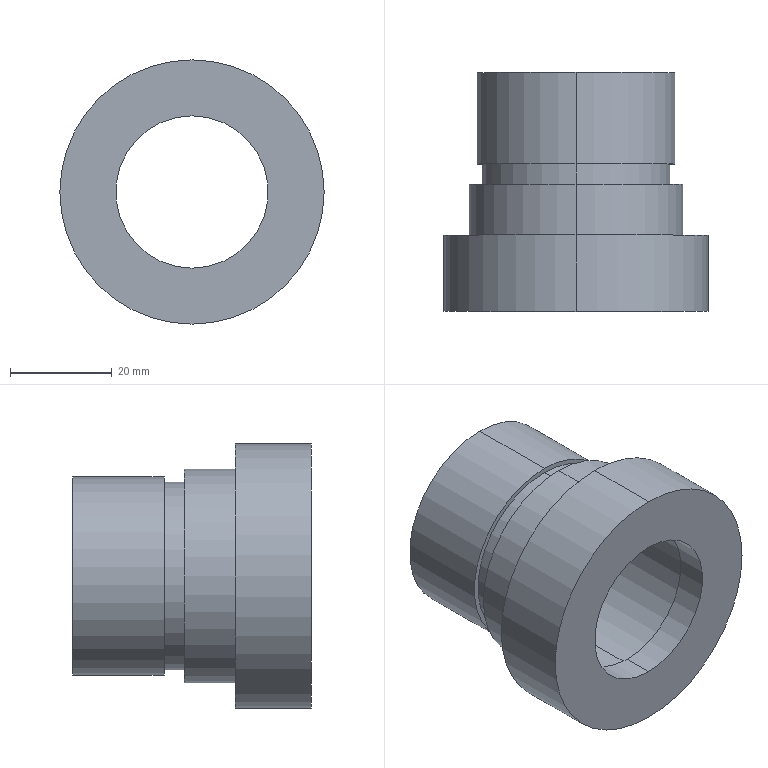Part | SolidWorks | features BaseBody 1 | 1 solid | 24 faces | box 52 x 47 x 52 mm | volume 34093 mm3 | cylinder 16 | plane 8 | commonest cylinder face diameters 32 x4 30 x2 35 x2 37 x2 39 x2 42 x2
STEP:
#1=CARTESIAN_POINT('',(0.,6.,-16.));
#2=VERTEX_POINT('',#1);
#3=CARTESIAN_POINT('',(0.,6.,16.));
#4=VERTEX_POINT('',#3);
#5=CARTESIAN_POINT('',(0.,6.,0.));
#6=DIRECTION('',(0.,1.,0.));
#7=DIRECTION('',(0.,0.,1.));
#8=AXIS2_PLACEMENT_3D('',#5,#6,#7);
#9=CIRCLE('',#8,16.);
#10=EDGE_CURVE('',#2,#4,#9,.T.);
#11=ORIENTED_EDGE('',*,*,#10,.F.);
#12=CARTESIAN_POINT('',(0.,41.,-16.));
#13=VERTEX_POINT('',#12);
#14=CARTESIAN_POINT('',(0.,6.,-16.));
#15=DIRECTION('',(0.,1.,0.));
#16=VECTOR('',#15,1000.);
#17=LINE('',#14,#16);
#18=EDGE_CURVE('',#2,#13,#17,.T.);
#19=ORIENTED_EDGE('',*,*,#18,.T.);
#20=CARTESIAN_POINT('',(0.,41.,16.));
#21=VERTEX_POINT('',#20);
#22=CARTESIAN_POINT('',(0.,41.,0.));
#23=DIRECTION('',(0.,-1.,0.));
#24=DIRECTION('',(0.,0.,1.));
#25=AXIS2_PLACEMENT_3D('',#22,#23,#24);
#26=CIRCLE('',#25,16.);
#27=EDGE_CURVE('',#21,#13,#26,.T.);
#28=ORIENTED_EDGE('',*,*,#27,.F.);
#29=CARTESIAN_POINT('',(0.,6.,16.));
#30=DIRECTION('',(0.,1.,0.));
#31=VECTOR('',#30,1000.);
#32=LINE('',#29,#31);
#33=EDGE_CURVE('',#4,#21,#32,.T.);
#34=ORIENTED_EDGE('',*,*,#33,.F.);
#35=EDGE_LOOP('',(#11,#19,#28,#34));
#36=FACE_OUTER_BOUND('',#35,.T.);
#37=CARTESIAN_POINT('',(0.,6.,0.));
#38=DIRECTION('',(0.,1.,0.));
#39=DIRECTION('',(0.,0.,1.));
#40=AXIS2_PLACEMENT_3D('',#37,#38,#39);
#41=CYLINDRICAL_SURFACE('',#40,16.);
#42=ADVANCED_FACE('',(#36),#41,.F.);
#43=CARTESIAN_POINT('',(0.,6.,15.));
#44=VERTEX_POINT('',#43);
#45=CARTESIAN_POINT('',(0.,6.,-15.));
#46=VERTEX_POINT('',#45);
#47=CARTESIAN_POINT('',(0.,6.,0.));
#48=DIRECTION('',(0.,-1.,0.));
#49=DIRECTION('',(0.,0.,-1.));
#50=AXIS2_PLACEMENT_3D('',#47,#48,#49);
#51=CIRCLE('',#50,15.);
#52=EDGE_CURVE('',#44,#46,#51,.T.);
#53=ORIENTED_EDGE('',*,*,#52,.F.);
#54=CARTESIAN_POINT('',(0.,0.,15.));
#55=VERTEX_POINT('',#54);
#56=CARTESIAN_POINT('',(0.,47.,15.));
#57=DIRECTION('',(0.,-1.,0.));
#58=VECTOR('',#57,1000.);
#59=LINE('',#56,#58);
#60=EDGE_CURVE('',#44,#55,#59,.T.);
#61=ORIENTED_EDGE('',*,*,#60,.T.);
#62=CARTESIAN_POINT('',(0.,0.,-15.));
#63=VERTEX_POINT('',#62);
#64=CARTESIAN_POINT('',(0.,0.,0.));
#65=DIRECTION('',(0.,1.,0.));
#66=DIRECTION('',(0.,0.,-1.));
#67=AXIS2_PLACEMENT_3D('',#64,#65,#66);
#68=CIRCLE('',#67,15.);
#69=EDGE_CURVE('',#63,#55,#68,.T.);
#70=ORIENTED_EDGE('',*,*,#69,.F.);
#71=CARTESIAN_POINT('',(0.,47.,-15.));
#72=DIRECTION('',(0.,-1.,0.));
#73=VECTOR('',#72,1000.);
#74=LINE('',#71,#73);
#75=EDGE_CURVE('',#46,#63,#74,.T.);
#76=ORIENTED_EDGE('',*,*,#75,.F.);
#77=EDGE_LOOP('',(#53,#61,#70,#76));
#78=FACE_OUTER_BOUND('',#77,.T.);
#79=CARTESIAN_POINT('',(0.,47.,0.));
#80=DIRECTION('',(0.,-1.,0.));
#81=DIRECTION('',(0.,0.,-1.));
#82=AXIS2_PLACEMENT_3D('',#79,#80,#81);
#83=CYLINDRICAL_SURFACE('',#82,15.);
#84=ADVANCED_FACE('',(#78),#83,.F.);
#85=CARTESIAN_POINT('',(0.,42.3,17.5));
#86=VERTEX_POINT('',#85);
#87=CARTESIAN_POINT('',(0.,42.3,-17.5));
#88=VERTEX_POINT('',#87);
#89=CARTESIAN_POINT('',(0.,42.3,0.));
#90=DIRECTION('',(0.,-1.,0.));
#91=DIRECTION('',(0.,0.,-1.));
#92=AXIS2_PLACEMENT_3D('',#89,#90,#91);
#93=CIRCLE('',#92,17.5);
#94=EDGE_CURVE('',#86,#88,#93,.T.);
#95=ORIENTED_EDGE('',*,*,#94,.F.);
#96=CARTESIAN_POINT('',(0.,41.,17.5));
#97=VERTEX_POINT('',#96);
#98=CARTESIAN_POINT('',(0.,42.3,17.5));
#99=DIRECTION('',(0.,-1.,0.));
#100=VECTOR('',#99,1000.);
#101=LINE('',#98,#100);
#102=EDGE_CURVE('',#86,#97,#101,.T.);
#103=ORIENTED_EDGE('',*,*,#102,.T.);
#104=CARTESIAN_POINT('',(0.,41.,-17.5));
#105=VERTEX_POINT('',#104);
#106=CARTESIAN_POINT('',(0.,41.,0.));
#107=DIRECTION('',(0.,1.,0.));
#108=DIRECTION('',(0.,0.,-1.));
#109=AXIS2_PLACEMENT_3D('',#106,#107,#108);
#110=CIRCLE('',#109,17.5);
#111=EDGE_CURVE('',#105,#97,#110,.T.);
#112=ORIENTED_EDGE('',*,*,#111,.F.);
#113=CARTESIAN_POINT('',(0.,42.3,-17.5));
#114=DIRECTION('',(0.,-1.,0.));
#115=VECTOR('',#114,1000.);
#116=LINE('',#113,#115);
#117=EDGE_CURVE('',#88,#105,#116,.T.);
#118=ORIENTED_EDGE('',*,*,#117,.F.);
#119=EDGE_LOOP('',(#95,#103,#112,#118));
#120=FACE_OUTER_BOUND('',#119,.T.);
#121=CARTESIAN_POINT('',(0.,42.3,0.));
#122=DIRECTION('',(0.,-1.,0.));
#123=DIRECTION('',(0.,0.,-1.));
#124=AXIS2_PLACEMENT_3D('',#121,#122,#123);
#125=CYLINDRICAL_SURFACE('',#124,17.5);
#126=ADVANCED_FACE('',(#120),#125,.F.);
#127=CARTESIAN_POINT('',(0.,15.,-26.));
#128=VERTEX_POINT('',#127);
#129=CARTESIAN_POINT('',(0.,15.,26.));
#130=VERTEX_POINT('',#129);
#131=CARTESIAN_POINT('',(0.,15.,0.));
#132=DIRECTION('',(0.,-1.,0.));
#133=DIRECTION('',(0.,0.,-1.));
#134=AXIS2_PLACEMENT_3D('',#131,#132,#133);
#135=CIRCLE('',#134,26.);
#136=EDGE_CURVE('',#128,#130,#135,.T.);
#137=ORIENTED_EDGE('',*,*,#136,.T.);
#138=CARTESIAN_POINT('',(0.,0.,26.));
#139=VERTEX_POINT('',#138);
#140=CARTESIAN_POINT('',(0.,47.,26.));
#141=DIRECTION('',(0.,-1.,0.));
#142=VECTOR('',#141,1000.);
#143=LINE('',#140,#142);
#144=EDGE_CURVE('',#130,#139,#143,.T.);
#145=ORIENTED_EDGE('',*,*,#144,.T.);
#146=CARTESIAN_POINT('',(0.,0.,-26.));
#147=VERTEX_POINT('',#146);
#148=CARTESIAN_POINT('',(0.,0.,0.));
#149=DIRECTION('',(0.,1.,0.));
#150=DIRECTION('',(0.,0.,-1.));
#151=AXIS2_PLACEMENT_3D('',#148,#149,#150);
#152=CIRCLE('',#151,26.);
#153=EDGE_CURVE('',#139,#147,#152,.T.);
#154=ORIENTED_EDGE('',*,*,#153,.T.);
#155=CARTESIAN_POINT('',(0.,47.,-26.));
#156=DIRECTION('',(0.,-1.,0.));
#157=VECTOR('',#156,1000.);
#158=LINE('',#155,#157);
#159=EDGE_CURVE('',#128,#147,#158,.T.);
#160=ORIENTED_EDGE('',*,*,#159,.F.);
#161=EDGE_LOOP('',(#137,#145,#154,#160));
#162=FACE_OUTER_BOUND('',#161,.T.);
#163=CARTESIAN_POINT('',(0.,47.,0.));
#164=DIRECTION('',(0.,-1.,0.));
#165=DIRECTION('',(0.,0.,-1.));
#166=AXIS2_PLACEMENT_3D('',#163,#164,#165);
#167=CYLINDRICAL_SURFACE('',#166,26.);
#168=ADVANCED_FACE('',(#162),#167,.T.);
#169=CARTESIAN_POINT('',(0.,42.3,16.));
#170=VERTEX_POINT('',#169);
#171=CARTESIAN_POINT('',(0.,42.3,-16.));
#172=VERTEX_POINT('',#171);
#173=CARTESIAN_POINT('',(0.,42.3,0.));
#174=DIRECTION('',(0.,-1.,0.));
#175=DIRECTION('',(0.,0.,1.));
#176=AXIS2_PLACEMENT_3D('',#173,#174,#175);
#177=CIRCLE('',#176,16.);
#178=EDGE_CURVE('',#170,#172,#177,.T.);
#179=ORIENTED_EDGE('',*,*,#178,.T.);
#180=CARTESIAN_POINT('',(0.,47.,-16.));
#181=VERTEX_POINT('',#180);
#182=CARTESIAN_POINT('',(0.,6.,-16.));
#183=DIRECTION('',(0.,1.,0.));
#184=VECTOR('',#183,1000.);
#185=LINE('',#182,#184);
#186=EDGE_CURVE('',#172,#181,#185,.T.);
#187=ORIENTED_EDGE('',*,*,#186,.T.);
#188=CARTESIAN_POINT('',(0.,47.,16.));
#189=VERTEX_POINT('',#188);
#190=CARTESIAN_POINT('',(0.,47.,0.));
#191=DIRECTION('',(0.,-1.,0.));
#192=DIRECTION('',(0.,0.,1.));
#193=AXIS2_PLACEMENT_3D('',#190,#191,#192);
#194=CIRCLE('',#193,16.);
#195=EDGE_CURVE('',#189,#181,#194,.T.);
#196=ORIENTED_EDGE('',*,*,#195,.F.);
#197=CARTESIAN_POINT('',(0.,6.,16.));
#198=DIRECTION('',(0.,1.,0.));
#199=VECTOR('',#198,1000.);
#200=LINE('',#197,#199);
#201=EDGE_CURVE('',#170,#189,#200,.T.);
#202=ORIENTED_EDGE('',*,*,#201,.F.);
#203=EDGE_LOOP('',(#179,#187,#196,#202));
#204=FACE_OUTER_BOUND('',#203,.T.);
#205=CARTESIAN_POINT('',(0.,6.,0.));
#206=DIRECTION('',(0.,1.,0.));
#207=DIRECTION('',(0.,0.,1.));
#208=AXIS2_PLACEMENT_3D('',#205,#206,#207);
#209=CYLINDRICAL_SURFACE('',#208,16.);
#210=ADVANCED_FACE('',(#204),#209,.F.);
#211=CARTESIAN_POINT('',(0.,15.,-21.));
#212=VERTEX_POINT('',#211);
#213=CARTESIAN_POINT('',(0.,15.,21.));
#214=VERTEX_POINT('',#213);
#215=CARTESIAN_POINT('',(0.,15.,0.));
#216=DIRECTION('',(0.,-1.,0.));
#217=DIRECTION('',(0.,0.,1.));
#218=AXIS2_PLACEMENT_3D('',#215,#216,#217);
#219=CIRCLE('',#218,21.);
#220=EDGE_CURVE('',#212,#214,#219,.T.);
#221=ORIENTED_EDGE('',*,*,#220,.F.);
#222=CARTESIAN_POINT('',(0.,25.,-21.));
#223=VERTEX_POINT('',#222);
#224=CARTESIAN_POINT('',(0.,15.,-21.));
#225=DIRECTION('',(0.,1.,0.));
#226=VECTOR('',#225,1000.);
#227=LINE('',#224,#226);
#228=EDGE_CURVE('',#212,#223,#227,.T.);
#229=ORIENTED_EDGE('',*,*,#228,.T.);
#230=CARTESIAN_POINT('',(0.,25.,21.));
#231=VERTEX_POINT('',#230);
#232=CARTESIAN_POINT('',(0.,25.,0.));
#233=DIRECTION('',(0.,-1.,0.));
#234=DIRECTION('',(0.,0.,1.));
#235=AXIS2_PLACEMENT_3D('',#232,#233,#234);
#236=CIRCLE('',#235,21.);
#237=EDGE_CURVE('',#223,#231,#236,.T.);
#238=ORIENTED_EDGE('',*,*,#237,.T.);
#239=CARTESIAN_POINT('',(0.,15.,21.));
#240=DIRECTION('',(0.,1.,0.));
#241=VECTOR('',#240,1000.);
#242=LINE('',#239,#241);
#243=EDGE_CURVE('',#214,#231,#242,.T.);
#244=ORIENTED_EDGE('',*,*,#243,.F.);
#245=EDGE_LOOP('',(#221,#229,#238,#244));
#246=FACE_OUTER_BOUND('',#245,.T.);
#247=CARTESIAN_POINT('',(0.,15.,0.));
#248=DIRECTION('',(0.,1.,0.));
#249=DIRECTION('',(0.,0.,1.));
#250=AXIS2_PLACEMENT_3D('',#247,#248,#249);
#251=CYLINDRICAL_SURFACE('',#250,21.);
#252=ADVANCED_FACE('',(#246),#251,.T.);
#253=CARTESIAN_POINT('',(0.,29.,19.5));
#254=VERTEX_POINT('',#253);
#255=CARTESIAN_POINT('',(0.,29.,-19.5));
#256=VERTEX_POINT('',#255);
#257=CARTESIAN_POINT('',(0.,29.,0.));
#258=DIRECTION('',(0.,1.,0.));
#259=DIRECTION('',(0.,0.,1.));
#260=AXIS2_PLACEMENT_3D('',#257,#258,#259);
#261=CIRCLE('',#260,19.5);
#262=EDGE_CURVE('',#254,#256,#261,.T.);
#263=ORIENTED_EDGE('',*,*,#262,.T.);
#264=CARTESIAN_POINT('',(0.,47.,-19.5));
#265=VERTEX_POINT('',#264);
#266=CARTESIAN_POINT('',(0.,25.,-19.5));
#267=DIRECTION('',(0.,1.,0.));
#268=VECTOR('',#267,1000.);
#269=LINE('',#266,#268);
#270=EDGE_CURVE('',#256,#265,#269,.T.);
#271=ORIENTED_EDGE('',*,*,#270,.T.);
#272=CARTESIAN_POINT('',(0.,47.,19.5));
#273=VERTEX_POINT('',#272);
#274=CARTESIAN_POINT('',(0.,47.,0.));
#275=DIRECTION('',(0.,1.,0.));
#276=DIRECTION('',(0.,0.,1.));
#277=AXIS2_PLACEMENT_3D('',#274,#275,#276);
#278=CIRCLE('',#277,19.5);
#279=EDGE_CURVE('',#273,#265,#278,.T.);
#280=ORIENTED_EDGE('',*,*,#279,.F.);
#281=CARTESIAN_POINT('',(0.,25.,19.5));
#282=DIRECTION('',(0.,1.,0.));
#283=VECTOR('',#282,1000.);
#284=LINE('',#281,#283);
#285=EDGE_CURVE('',#254,#273,#284,.T.);
#286=ORIENTED_EDGE('',*,*,#285,.F.);
#287=EDGE_LOOP('',(#263,#271,#280,#286));
#288=FACE_OUTER_BOUND('',#287,.T.);
#289=CARTESIAN_POINT('',(0.,25.,0.));
#290=DIRECTION('',(0.,1.,0.));
#291=DIRECTION('',(0.,0.,1.));
#292=AXIS2_PLACEMENT_3D('',#289,#290,#291);
#293=CYLINDRICAL_SURFACE('',#292,19.5);
#294=ADVANCED_FACE('',(#288),#293,.T.);
#295=CARTESIAN_POINT('',(0.,25.,-18.5));
#296=VERTEX_POINT('',#295);
#297=CARTESIAN_POINT('',(0.,25.,18.5));
#298=VERTEX_POINT('',#297);
#299=CARTESIAN_POINT('',(0.,25.,0.));
#300=DIRECTION('',(0.,-1.,0.));
#301=DIRECTION('',(0.,0.,1.));
#302=AXIS2_PLACEMENT_3D('',#299,#300,#301);
#303=CIRCLE('',#302,18.5);
#304=EDGE_CURVE('',#296,#298,#303,.T.);
#305=ORIENTED_EDGE('',*,*,#304,.F.);
#306=CARTESIAN_POINT('',(0.,29.,-18.5));
#307=VERTEX_POINT('',#306);
#308=CARTESIAN_POINT('',(0.,25.,-18.5));
#309=DIRECTION('',(0.,1.,0.));
#310=VECTOR('',#309,1000.);
#311=LINE('',#308,#310);
#312=EDGE_CURVE('',#296,#307,#311,.T.);
#313=ORIENTED_EDGE('',*,*,#312,.T.);
#314=CARTESIAN_POINT('',(0.,29.,18.5));
#315=VERTEX_POINT('',#314);
#316=CARTESIAN_POINT('',(0.,29.,0.));
#317=DIRECTION('',(0.,-1.,0.));
#318=DIRECTION('',(0.,0.,1.));
#319=AXIS2_PLACEMENT_3D('',#316,#317,#318);
#320=CIRCLE('',#319,18.5);
#321=EDGE_CURVE('',#307,#315,#320,.T.);
#322=ORIENTED_EDGE('',*,*,#321,.T.);
#323=CARTESIAN_POINT('',(0.,25.,18.5));
#324=DIRECTION('',(0.,1.,0.));
#325=VECTOR('',#324,1000.);
#326=LINE('',#323,#325);
#327=EDGE_CURVE('',#298,#315,#326,.T.);
#328=ORIENTED_EDGE('',*,*,#327,.F.);
#329=EDGE_LOOP('',(#305,#313,#322,#328));
#330=FACE_OUTER_BOUND('',#329,.T.);
#331=CARTESIAN_POINT('',(0.,25.,0.));
#332=DIRECTION('',(0.,1.,0.));
#333=DIRECTION('',(0.,0.,1.));
#334=AXIS2_PLACEMENT_3D('',#331,#332,#333);
#335=CYLINDRICAL_SURFACE('',#334,18.5);
#336=ADVANCED_FACE('',(#330),#335,.T.);
#337=ORIENTED_EDGE('',*,*,#18,.F.);
#338=CARTESIAN_POINT('',(0.,6.,0.));
#339=DIRECTION('',(0.,1.,0.));
#340=DIRECTION('',(0.,0.,1.));
#341=AXIS2_PLACEMENT_3D('',#338,#339,#340);
#342=CIRCLE('',#341,16.);
#343=EDGE_CURVE('',#4,#2,#342,.T.);
#344=ORIENTED_EDGE('',*,*,#343,.F.);
#345=ORIENTED_EDGE('',*,*,#33,.T.);
#346=CARTESIAN_POINT('',(0.,41.,0.));
#347=DIRECTION('',(0.,-1.,0.));
#348=DIRECTION('',(0.,0.,1.));
#349=AXIS2_PLACEMENT_3D('',#346,#347,#348);
#350=CIRCLE('',#349,16.);
#351=EDGE_CURVE('',#13,#21,#350,.T.);
#352=ORIENTED_EDGE('',*,*,#351,.F.);
#353=EDGE_LOOP('',(#337,#344,#345,#352));
#354=FACE_OUTER_BOUND('',#353,.T.);
#355=CARTESIAN_POINT('',(0.,6.,0.));
#356=DIRECTION('',(0.,1.,0.));
#357=DIRECTION('',(0.,0.,1.));
#358=AXIS2_PLACEMENT_3D('',#355,#356,#357);
#359=CYLINDRICAL_SURFACE('',#358,16.);
#360=ADVANCED_FACE('',(#354),#359,.F.);
#361=ORIENTED_EDGE('',*,*,#343,.T.);
#362=ORIENTED_EDGE('',*,*,#10,.T.);
#363=EDGE_LOOP('',(#361,#362));
#364=FACE_OUTER_BOUND('',#363,.T.);
#365=CARTESIAN_POINT('',(0.,6.,0.));
#366=DIRECTION('',(0.,-1.,0.));
#367=DIRECTION('',(0.,0.,-1.));
#368=AXIS2_PLACEMENT_3D('',#365,#366,#367);
#369=CIRCLE('',#368,15.);
#370=EDGE_CURVE('',#46,#44,#369,.T.);
#371=ORIENTED_EDGE('',*,*,#370,.T.);
#372=ORIENTED_EDGE('',*,*,#52,.T.);
#373=EDGE_LOOP('',(#371,#372));
#374=FACE_BOUND('',#373,.T.);
#375=CARTESIAN_POINT('',(0.,6.,0.));
#376=DIRECTION('',(0.,1.,0.));
#377=DIRECTION('',(0.,0.,1.));
#378=AXIS2_PLACEMENT_3D('',#375,#376,#377);
#379=PLANE('',#378);
#380=ADVANCED_FACE('',(#364,#374),#379,.T.);
#381=ORIENTED_EDGE('',*,*,#27,.T.);
#382=ORIENTED_EDGE('',*,*,#351,.T.);
#383=EDGE_LOOP('',(#381,#382));
#384=FACE_BOUND('',#383,.T.);
#385=ORIENTED_EDGE('',*,*,#111,.T.);
#386=CARTESIAN_POINT('',(0.,41.,0.));
#387=DIRECTION('',(0.,1.,0.));
#388=DIRECTION('',(0.,0.,-1.));
#389=AXIS2_PLACEMENT_3D('',#386,#387,#388);
#390=CIRCLE('',#389,17.5);
#391=EDGE_CURVE('',#97,#105,#390,.T.);
#392=ORIENTED_EDGE('',*,*,#391,.T.);
#393=EDGE_LOOP('',(#385,#392));
#394=FACE_OUTER_BOUND('',#393,.T.);
#395=CARTESIAN_POINT('',(0.,41.,0.));
#396=DIRECTION('',(0.,1.,0.));
#397=DIRECTION('',(0.,0.,1.));
#398=AXIS2_PLACEMENT_3D('',#395,#396,#397);
#399=PLANE('',#398);
#400=ADVANCED_FACE('',(#384,#394),#399,.T.);
#401=ORIENTED_EDGE('',*,*,#60,.F.);
#402=ORIENTED_EDGE('',*,*,#370,.F.);
#403=ORIENTED_EDGE('',*,*,#75,.T.);
#404=CARTESIAN_POINT('',(0.,0.,0.));
#405=DIRECTION('',(0.,1.,0.));
#406=DIRECTION('',(0.,0.,-1.));
#407=AXIS2_PLACEMENT_3D('',#404,#405,#406);
#408=CIRCLE('',#407,15.);
#409=EDGE_CURVE('',#55,#63,#408,.T.);
#410=ORIENTED_EDGE('',*,*,#409,.F.);
#411=EDGE_LOOP('',(#401,#402,#403,#410));
#412=FACE_OUTER_BOUND('',#411,.T.);
#413=CARTESIAN_POINT('',(0.,47.,0.));
#414=DIRECTION('',(0.,-1.,0.));
#415=DIRECTION('',(0.,0.,-1.));
#416=AXIS2_PLACEMENT_3D('',#413,#414,#415);
#417=CYLINDRICAL_SURFACE('',#416,15.);
#418=ADVANCED_FACE('',(#412),#417,.F.);
#419=ORIENTED_EDGE('',*,*,#102,.F.);
#420=CARTESIAN_POINT('',(0.,42.3,0.));
#421=DIRECTION('',(0.,-1.,0.));
#422=DIRECTION('',(0.,0.,-1.));
#423=AXIS2_PLACEMENT_3D('',#420,#421,#422);
#424=CIRCLE('',#423,17.5);
#425=EDGE_CURVE('',#88,#86,#424,.T.);
#426=ORIENTED_EDGE('',*,*,#425,.F.);
#427=ORIENTED_EDGE('',*,*,#117,.T.);
#428=ORIENTED_EDGE('',*,*,#391,.F.);
#429=EDGE_LOOP('',(#419,#426,#427,#428));
#430=FACE_OUTER_BOUND('',#429,.T.);
#431=CARTESIAN_POINT('',(0.,42.3,0.));
#432=DIRECTION('',(0.,-1.,0.));
#433=DIRECTION('',(0.,0.,-1.));
#434=AXIS2_PLACEMENT_3D('',#431,#432,#433);
#435=CYLINDRICAL_SURFACE('',#434,17.5);
#436=ADVANCED_FACE('',(#430),#435,.F.);
#437=ORIENTED_EDGE('',*,*,#69,.T.);
#438=ORIENTED_EDGE('',*,*,#409,.T.);
#439=EDGE_LOOP('',(#437,#438));
#440=FACE_BOUND('',#439,.T.);
#441=CARTESIAN_POINT('',(0.,0.,0.));
#442=DIRECTION('',(0.,1.,0.));
#443=DIRECTION('',(0.,0.,-1.));
#444=AXIS2_PLACEMENT_3D('',#441,#442,#443);
#445=CIRCLE('',#444,26.);
#446=EDGE_CURVE('',#147,#139,#445,.T.);
#447=ORIENTED_EDGE('',*,*,#446,.F.);
#448=ORIENTED_EDGE('',*,*,#153,.F.);
#449=EDGE_LOOP('',(#447,#448));
#450=FACE_OUTER_BOUND('',#449,.T.);
#451=CARTESIAN_POINT('',(0.,0.,0.));
#452=DIRECTION('',(0.,1.,0.));
#453=DIRECTION('',(0.,0.,1.));
#454=AXIS2_PLACEMENT_3D('',#451,#452,#453);
#455=PLANE('',#454);
#456=ADVANCED_FACE('',(#440,#450),#455,.F.);
#457=ORIENTED_EDGE('',*,*,#178,.F.);
#458=CARTESIAN_POINT('',(0.,42.3,0.));
#459=DIRECTION('',(0.,-1.,0.));
#460=DIRECTION('',(0.,0.,1.));
#461=AXIS2_PLACEMENT_3D('',#458,#459,#460);
#462=CIRCLE('',#461,16.);
#463=EDGE_CURVE('',#172,#170,#462,.T.);
#464=ORIENTED_EDGE('',*,*,#463,.F.);
#465=EDGE_LOOP('',(#457,#464));
#466=FACE_BOUND('',#465,.T.);
#467=ORIENTED_EDGE('',*,*,#425,.T.);
#468=ORIENTED_EDGE('',*,*,#94,.T.);
#469=EDGE_LOOP('',(#467,#468));
#470=FACE_OUTER_BOUND('',#469,.T.);
#471=CARTESIAN_POINT('',(0.,42.3,0.));
#472=DIRECTION('',(0.,1.,0.));
#473=DIRECTION('',(0.,0.,1.));
#474=AXIS2_PLACEMENT_3D('',#471,#472,#473);
#475=PLANE('',#474);
#476=ADVANCED_FACE('',(#466,#470),#475,.F.);
#477=ORIENTED_EDGE('',*,*,#144,.F.);
#478=CARTESIAN_POINT('',(0.,15.,0.));
#479=DIRECTION('',(0.,-1.,0.));
#480=DIRECTION('',(0.,0.,-1.));
#481=AXIS2_PLACEMENT_3D('',#478,#479,#480);
#482=CIRCLE('',#481,26.);
#483=EDGE_CURVE('',#130,#128,#482,.T.);
#484=ORIENTED_EDGE('',*,*,#483,.T.);
#485=ORIENTED_EDGE('',*,*,#159,.T.);
#486=ORIENTED_EDGE('',*,*,#446,.T.);
#487=EDGE_LOOP('',(#477,#484,#485,#486));
#488=FACE_OUTER_BOUND('',#487,.T.);
#489=CARTESIAN_POINT('',(0.,47.,0.));
#490=DIRECTION('',(0.,-1.,0.));
#491=DIRECTION('',(0.,0.,-1.));
#492=AXIS2_PLACEMENT_3D('',#489,#490,#491);
#493=CYLINDRICAL_SURFACE('',#492,26.);
#494=ADVANCED_FACE('',(#488),#493,.T.);
#495=ORIENTED_EDGE('',*,*,#186,.F.);
#496=ORIENTED_EDGE('',*,*,#463,.T.);
#497=ORIENTED_EDGE('',*,*,#201,.T.);
#498=CARTESIAN_POINT('',(0.,47.,0.));
#499=DIRECTION('',(0.,-1.,0.));
#500=DIRECTION('',(0.,0.,1.));
#501=AXIS2_PLACEMENT_3D('',#498,#499,#500);
#502=CIRCLE('',#501,16.);
#503=EDGE_CURVE('',#181,#189,#502,.T.);
#504=ORIENTED_EDGE('',*,*,#503,.F.);
#505=EDGE_LOOP('',(#495,#496,#497,#504));
#506=FACE_OUTER_BOUND('',#505,.T.);
#507=CARTESIAN_POINT('',(0.,6.,0.));
#508=DIRECTION('',(0.,1.,0.));
#509=DIRECTION('',(0.,0.,1.));
#510=AXIS2_PLACEMENT_3D('',#507,#508,#509);
#511=CYLINDRICAL_SURFACE('',#510,16.);
#512=ADVANCED_FACE('',(#506),#511,.F.);
#513=ORIENTED_EDGE('',*,*,#136,.F.);
#514=ORIENTED_EDGE('',*,*,#483,.F.);
#515=EDGE_LOOP('',(#513,#514));
#516=FACE_OUTER_BOUND('',#515,.T.);
#517=CARTESIAN_POINT('',(0.,15.,0.));
#518=DIRECTION('',(0.,-1.,0.));
#519=DIRECTION('',(0.,0.,1.));
#520=AXIS2_PLACEMENT_3D('',#517,#518,#519);
#521=CIRCLE('',#520,21.);
#522=EDGE_CURVE('',#214,#212,#521,.T.);
#523=ORIENTED_EDGE('',*,*,#522,.T.);
#524=ORIENTED_EDGE('',*,*,#220,.T.);
#525=EDGE_LOOP('',(#523,#524));
#526=FACE_BOUND('',#525,.T.);
#527=CARTESIAN_POINT('',(0.,15.,0.));
#528=DIRECTION('',(0.,1.,0.));
#529=DIRECTION('',(0.,0.,1.));
#530=AXIS2_PLACEMENT_3D('',#527,#528,#529);
#531=PLANE('',#530);
#532=ADVANCED_FACE('',(#516,#526),#531,.T.);
#533=ORIENTED_EDGE('',*,*,#279,.T.);
#534=CARTESIAN_POINT('',(0.,47.,0.));
#535=DIRECTION('',(0.,1.,0.));
#536=DIRECTION('',(0.,0.,1.));
#537=AXIS2_PLACEMENT_3D('',#534,#535,#536);
#538=CIRCLE('',#537,19.5);
#539=EDGE_CURVE('',#265,#273,#538,.T.);
#540=ORIENTED_EDGE('',*,*,#539,.T.);
#541=EDGE_LOOP('',(#533,#540));
#542=FACE_OUTER_BOUND('',#541,.T.);
#543=ORIENTED_EDGE('',*,*,#195,.T.);
#544=ORIENTED_EDGE('',*,*,#503,.T.);
#545=EDGE_LOOP('',(#543,#544));
#546=FACE_BOUND('',#545,.T.);
#547=CARTESIAN_POINT('',(0.,47.,0.));
#548=DIRECTION('',(0.,1.,0.));
#549=DIRECTION('',(0.,0.,1.));
#550=AXIS2_PLACEMENT_3D('',#547,#548,#549);
#551=PLANE('',#550);
#552=ADVANCED_FACE('',(#542,#546),#551,.T.);
#553=ORIENTED_EDGE('',*,*,#228,.F.);
#554=ORIENTED_EDGE('',*,*,#522,.F.);
#555=ORIENTED_EDGE('',*,*,#243,.T.);
#556=CARTESIAN_POINT('',(0.,25.,0.));
#557=DIRECTION('',(0.,-1.,0.));
#558=DIRECTION('',(0.,0.,1.));
#559=AXIS2_PLACEMENT_3D('',#556,#557,#558);
#560=CIRCLE('',#559,21.);
#561=EDGE_CURVE('',#231,#223,#560,.T.);
#562=ORIENTED_EDGE('',*,*,#561,.T.);
#563=EDGE_LOOP('',(#553,#554,#555,#562));
#564=FACE_OUTER_BOUND('',#563,.T.);
#565=CARTESIAN_POINT('',(0.,15.,0.));
#566=DIRECTION('',(0.,1.,0.));
#567=DIRECTION('',(0.,0.,1.));
#568=AXIS2_PLACEMENT_3D('',#565,#566,#567);
#569=CYLINDRICAL_SURFACE('',#568,21.);
#570=ADVANCED_FACE('',(#564),#569,.T.);
#571=ORIENTED_EDGE('',*,*,#270,.F.);
#572=CARTESIAN_POINT('',(0.,29.,0.));
#573=DIRECTION('',(0.,1.,0.));
#574=DIRECTION('',(0.,0.,1.));
#575=AXIS2_PLACEMENT_3D('',#572,#573,#574);
#576=CIRCLE('',#575,19.5);
#577=EDGE_CURVE('',#256,#254,#576,.T.);
#578=ORIENTED_EDGE('',*,*,#577,.T.);
#579=ORIENTED_EDGE('',*,*,#285,.T.);
#580=ORIENTED_EDGE('',*,*,#539,.F.);
#581=EDGE_LOOP('',(#571,#578,#579,#580));
#582=FACE_OUTER_BOUND('',#581,.T.);
#583=CARTESIAN_POINT('',(0.,25.,0.));
#584=DIRECTION('',(0.,1.,0.));
#585=DIRECTION('',(0.,0.,1.));
#586=AXIS2_PLACEMENT_3D('',#583,#584,#585);
#587=CYLINDRICAL_SURFACE('',#586,19.5);
#588=ADVANCED_FACE('',(#582),#587,.T.);
#589=CARTESIAN_POINT('',(0.,25.,0.));
#590=DIRECTION('',(0.,-1.,0.));
#591=DIRECTION('',(0.,0.,1.));
#592=AXIS2_PLACEMENT_3D('',#589,#590,#591);
#593=CIRCLE('',#592,18.5);
#594=EDGE_CURVE('',#298,#296,#593,.T.);
#595=ORIENTED_EDGE('',*,*,#594,.T.);
#596=ORIENTED_EDGE('',*,*,#304,.T.);
#597=EDGE_LOOP('',(#595,#596));
#598=FACE_BOUND('',#597,.T.);
#599=ORIENTED_EDGE('',*,*,#561,.F.);
#600=ORIENTED_EDGE('',*,*,#237,.F.);
#601=EDGE_LOOP('',(#599,#600));
#602=FACE_OUTER_BOUND('',#601,.T.);
#603=CARTESIAN_POINT('',(0.,25.,0.));
#604=DIRECTION('',(0.,1.,0.));
#605=DIRECTION('',(0.,0.,1.));
#606=AXIS2_PLACEMENT_3D('',#603,#604,#605);
#607=PLANE('',#606);
#608=ADVANCED_FACE('',(#598,#602),#607,.T.);
#609=CARTESIAN_POINT('',(0.,29.,0.));
#610=DIRECTION('',(0.,-1.,0.));
#611=DIRECTION('',(0.,0.,1.));
#612=AXIS2_PLACEMENT_3D('',#609,#610,#611);
#613=CIRCLE('',#612,18.5);
#614=EDGE_CURVE('',#315,#307,#613,.T.);
#615=ORIENTED_EDGE('',*,*,#614,.F.);
#616=ORIENTED_EDGE('',*,*,#321,.F.);
#617=EDGE_LOOP('',(#615,#616));
#618=FACE_BOUND('',#617,.T.);
#619=ORIENTED_EDGE('',*,*,#262,.F.);
#620=ORIENTED_EDGE('',*,*,#577,.F.);
#621=EDGE_LOOP('',(#619,#620));
#622=FACE_OUTER_BOUND('',#621,.T.);
#623=CARTESIAN_POINT('',(0.,29.,0.));
#624=DIRECTION('',(0.,1.,0.));
#625=DIRECTION('',(0.,0.,1.));
#626=AXIS2_PLACEMENT_3D('',#623,#624,#625);
#627=PLANE('',#626);
#628=ADVANCED_FACE('',(#618,#622),#627,.F.);
#629=ORIENTED_EDGE('',*,*,#312,.F.);
#630=ORIENTED_EDGE('',*,*,#594,.F.);
#631=ORIENTED_EDGE('',*,*,#327,.T.);
#632=ORIENTED_EDGE('',*,*,#614,.T.);
#633=EDGE_LOOP('',(#629,#630,#631,#632));
#634=FACE_OUTER_BOUND('',#633,.T.);
#635=CARTESIAN_POINT('',(0.,25.,0.));
#636=DIRECTION('',(0.,1.,0.));
#637=DIRECTION('',(0.,0.,1.));
#638=AXIS2_PLACEMENT_3D('',#635,#636,#637);
#639=CYLINDRICAL_SURFACE('',#638,18.5);
#640=ADVANCED_FACE('',(#634),#639,.T.);
#641=CLOSED_SHELL('',(#42,#84,#126,#168,#210,#252,#294,#336,#360,#380,#400,#418,#436,#456,#476,#494,#512,#532,#552,#570,#588,#608,#628,#640));
#642=MANIFOLD_SOLID_BREP('',#641);
#643=CARTESIAN_POINT('',(0.,0.,0.));
#644=DIRECTION('',(0.,0.,1.));
#645=DIRECTION('',(1.,0.,0.));
#646=AXIS2_PLACEMENT_3D('',#643,#644,#645);
#647=(LENGTH_UNIT()NAMED_UNIT(*)SI_UNIT(.MILLI.,.METRE.));
#648=UNCERTAINTY_MEASURE_WITH_UNIT(LENGTH_MEASURE(0.00001),#647,'','');
#649=(NAMED_UNIT(*)PLANE_ANGLE_UNIT()SI_UNIT($,.RADIAN.));
#650=(NAMED_UNIT(*)SI_UNIT($,.STERADIAN.)SOLID_ANGLE_UNIT());
#651=(GEOMETRIC_REPRESENTATION_CONTEXT(3)GLOBAL_UNCERTAINTY_ASSIGNED_CONTEXT((#648))GLOBAL_UNIT_ASSIGNED_CONTEXT((#647,#649,#650))REPRESENTATION_CONTEXT('',''));
#652=ADVANCED_BREP_SHAPE_REPRESENTATION('',(#642,#646),#651);